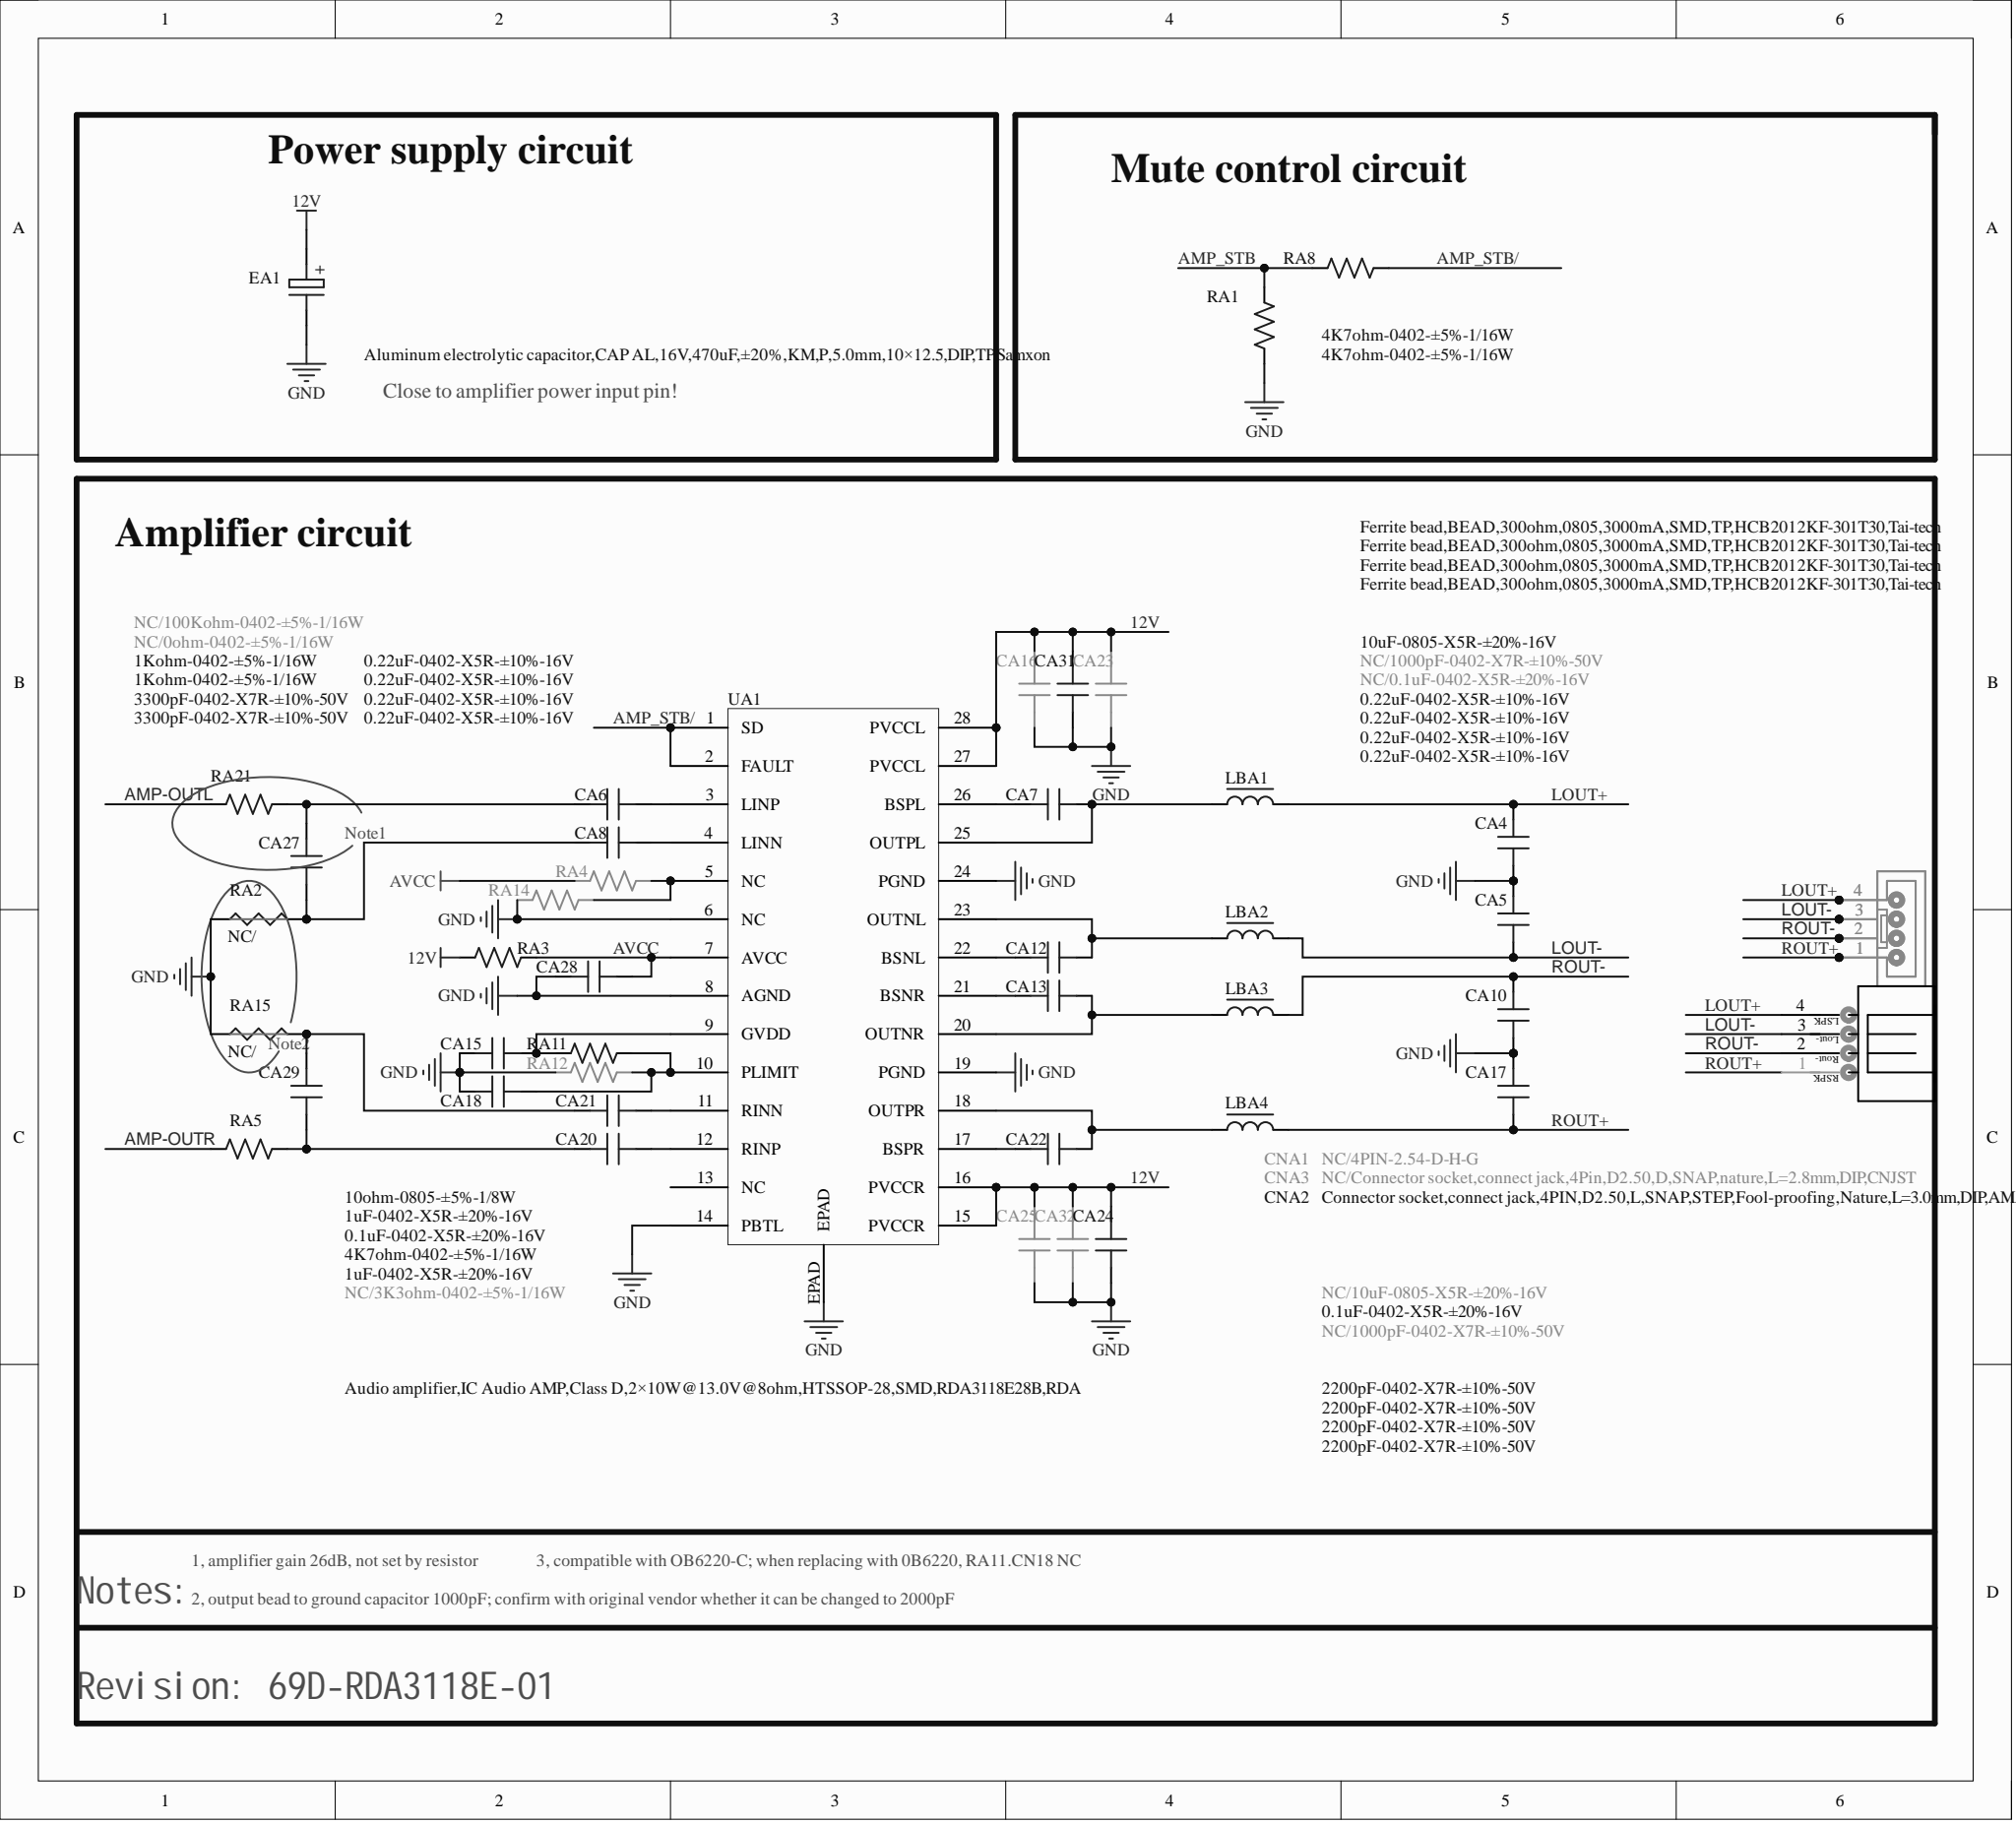Circuit board | Altium Designer | 574 parts | 274 nets | one sheet of the schematic
Parts on this sheet (reference | value | footprint):
CA4 | 2200pF-0402-X7R-±10%-50V | C0402
CA5 | 2200pF-0402-X7R-±10%-50V | C0402
CA6 | 0.22uF-0402-X5R-±10%-16V | C0402
CA7 | 0.22uF-0402-X5R-±10%-16V | C0402
CA8 | 0.22uF-0402-X5R-±10%-16V | C0402
CA10 | 2200pF-0402-X7R-±10%-50V | C0402
CA12 | 0.22uF-0402-X5R-±10%-16V | C0402
CA13 | 0.22uF-0402-X5R-±10%-16V | C0402
CA15 | 0.1uF-0402-X5R-±20%-16V | C0402
CA16 | NC/1000pF-0402-X7R-±10%-50V | C0402
CA17 | 2200pF-0402-X7R-±10%-50V | C0402
CA18 | 1uF-0402-X5R-±20%-16V | C0402
CA20 | 0.22uF-0402-X5R-±10%-16V | C0402
CA21 | 0.22uF-0402-X5R-±10%-16V | C0402
CA22 | 0.22uF-0402-X5R-±10%-16V | C0402
CA23 | NC/0.1uF-0402-X5R-±20%-16V | C0402
CA24 | 0.1uF-0402-X5R-±20%-16V | C0402
CA25 | NC/1000pF-0402-X7R-±10%-50V | C0402
CA27 | 3300pF-0402-X7R-±10%-50V | C0402
CA28 | 1uF-0402-X5R-±20%-16V | C0402
CA29 | 3300pF-0402-X7R-±10%-50V | C0402
CA31 | 10uF-0805-X5R-±20%-16V | C0805
CA32 | NC/10uF-0805-X5R-±20%-16V | C0805
CNA1 | NC/4PIN-2.54-D-H-G | SIP4/2.54D-1
CNA2 | Connector socket,connect jack,4PIN,D2.50,L,SNAP,STEP,Fool-proofing,Nature,L=3.0mm,DIP,AMA | SIP4H/2.54D-2
CNA3 | NC/Connector socket,connect jack,4Pin,D2.50,D,SNAP,nature,L=2.8mm,DIP,CNJST | SIP4/2.5D-2
EA1 | Aluminum electrolytic capacitor,CAP AL,16V,470uF,±20%,KM,P,5.0mm,10×12.5,DIP,TP,Samxon | EC(10*12.5)-V-5
LBA1 | Ferrite bead,BEAD,300ohm,0805,3000mA,SMD,TP,HCB2012KF-301T30,Tai-tech | L0805
LBA2 | Ferrite bead,BEAD,300ohm,0805,3000mA,SMD,TP,HCB2012KF-301T30,Tai-tech | L0805
LBA3 | Ferrite bead,BEAD,300ohm,0805,3000mA,SMD,TP,HCB2012KF-301T30,Tai-tech | L0805
LBA4 | Ferrite bead,BEAD,300ohm,0805,3000mA,SMD,TP,HCB2012KF-301T30,Tai-tech | L0805
RA1 | 4K7ohm-0402-±5%-1/16W | R0402
RA2 | NC/ | GND
RA3 | 10ohm-0805-±5%-1/8W | R0805
RA4 | NC/100Kohm-0402-±5%-1/16W | R0402
RA5 | 1Kohm-0402-±5%-1/16W | R0402
RA8 | 4K7ohm-0402-±5%-1/16W | R0402
RA11 | 4K7ohm-0402-±5%-1/16W | R0402
RA12 | NC/3K3ohm-0402-±5%-1/16W | R0402
RA14 | NC/0ohm-0402-±5%-1/16W | R0402
RA15 | NC/ | GND
RA21 | 1Kohm-0402-±5%-1/16W | R0402
UA1 | Audio amplifier,IC Audio AMP,Class D,2×10W@13.0V@8ohm,HTSSOP-28,SMD,RDA3118E28B,RDA | SSOP28/0.65-5
Nets of these parts (net: part-pin ...):
ROUT-: CA10-1 CNA1-2 CNA2-2 CNA3-2 LBA3-2
ROUT+: CA17-2 CNA1-1 CNA2-1 CNA3-1 LBA4-2
NetRA4_1: RA4-1 RA14-2 UA1-5
NetCA22_2: CA22-2 LBA4-1 UA1-18
NetCA22_1: CA22-1 UA1-17
NetCA21_2: CA21-2 CA29-2 RA15-JP_1K
NetCA21_1: CA21-1 UA1-11
NetCA20_2: CA20-2 CA29-1 RA5-2
NetCA20_1: CA20-1 UA1-12
NetCA18_1: CA18-1 RA11-1 RA12-1 UA1-10
NetCA15_1: CA15-1 RA11-2 UA1-9
NetCA13_2: CA13-2 LBA3-1 UA1-20
NetCA13_1: CA13-1 UA1-21
NetCA12_2: CA12-2 LBA2-1 UA1-23
NetCA12_1: CA12-1 UA1-22
NetCA8_2: CA8-2 CA27-2 RA2-JP_1K
NetCA8_1: CA8-1 UA1-4
NetCA7_2: CA7-2 LBA1-1 UA1-25
NetCA7_1: CA7-1 UA1-26
NetCA6_2: CA6-2 CA27-1 RA21-2
NetCA6_1: CA6-1 UA1-3
LOUT-: CA5-1 CNA1-3 CNA2-3 CNA3-3 LBA2-2
LOUT+: CA4-1 CNA1-4 CNA2-4 CNA3-4 LBA1-2
GND: CA4-2 CA5-2 CA10-2 CA15-2 CA16-1 CA17-1 CA18-2 CA23-1 CA24-1 CA25-1 CA28-1 CA31-1 CA32-1 EA1-2 RA1-1 RA2-JP_2K RA12-2 RA14-1 RA15-JP_2K UA1-6 UA1-8 UA1-14 UA1-19 UA1-24 UA1-EPAD
AVCC: CA28-2 RA3-2 RA4-2 UA1-7
AMP_STB/: RA8-2 UA1-1 UA1-2
AMP_STB: RA1-2 RA8-1
AMP-OUTR: RA5-1
AMP-OUTL: RA21-1
12V: CA16-2 CA23-2 CA24-2 CA25-2 CA31-2 CA32-2 EA1-1 RA3-1 UA1-15 UA1-16 UA1-27 UA1-28